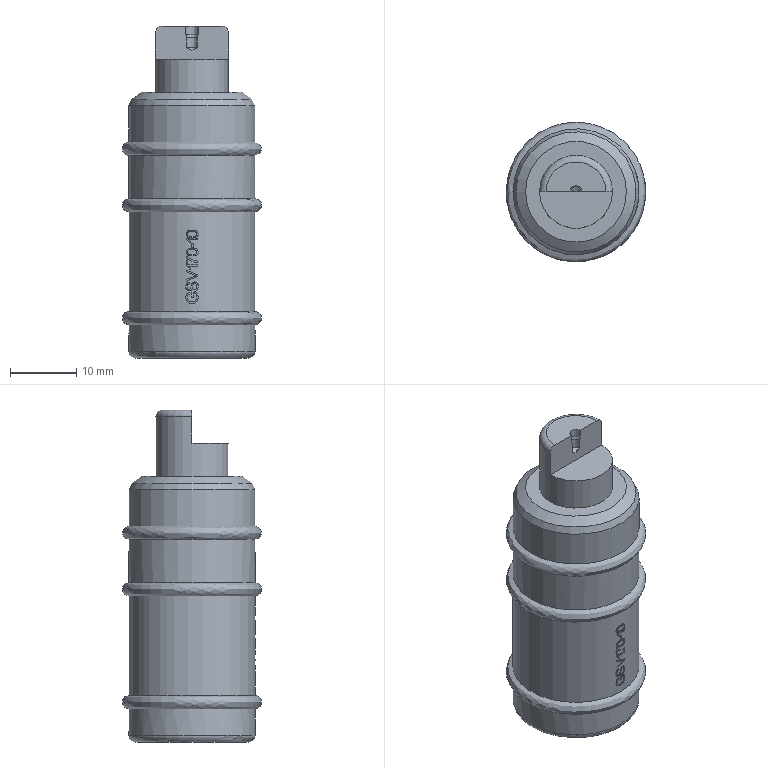Part | NX | features solid 2 | 1 solid | 142 faces | box 21 x 21 x 50 mm | volume 12025 mm3 | plane 72 | cylinder 59 | cone 6 | spline 3 | torus 2 | commonest cylinder face diameters 18.8 x9 19 x6 0.759 x2 0.906 x2 0.909 x2 0.919 x2